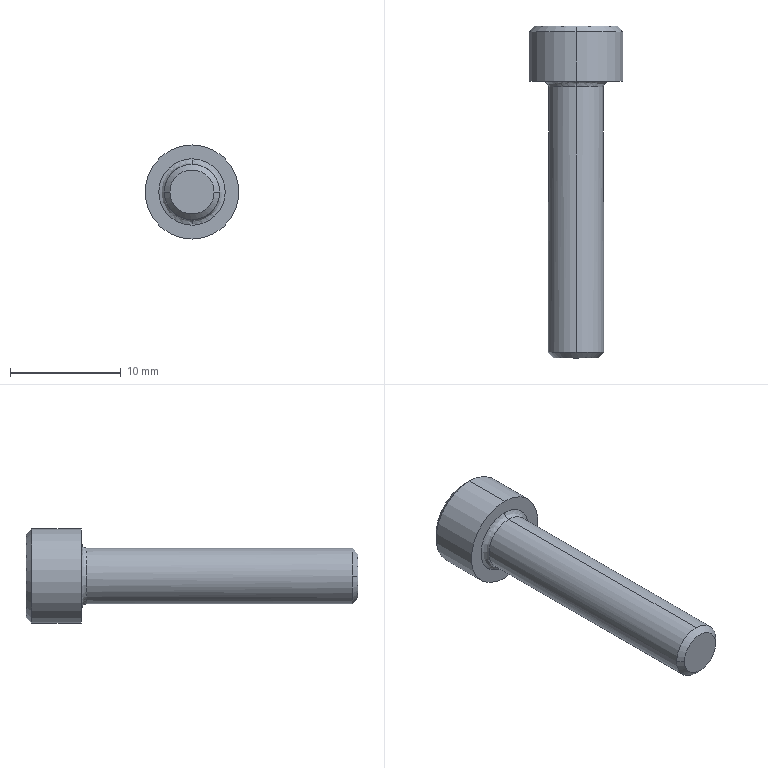Part | STEP file | 1 solid | 20 faces | box 8.5 x 30 x 8.5 mm | volume 734.47 mm3 | plane 10 | cone 4 | cylinder 4 | spline 2 | commonest cylinder face diameters 5 x2 8.5 x2